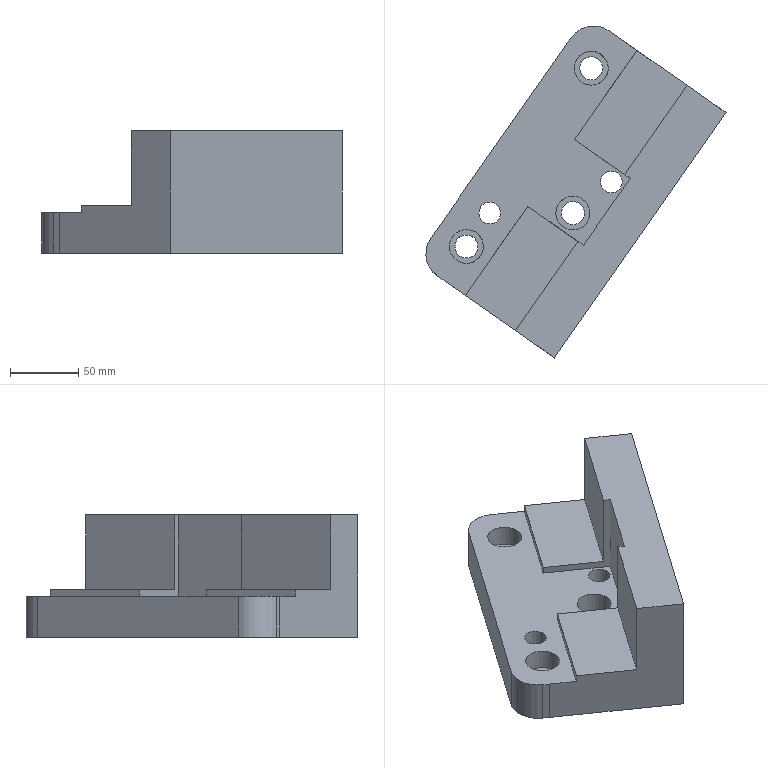Part | NX | features solid 2 | 1 solid | 35 faces | box 220.726 x 244.056 x 90 mm | volume 1242113 mm3 | plane 23 | cylinder 12 | commonest cylinder face diameters 17 x3 25 x3 16 x2 20 x2 40 x2
STEP:
#1=CARTESIAN_POINT('',(39.998,94.071,-429.059));
#2=VERTEX_POINT('',#1);
#3=CARTESIAN_POINT('',(3.136,119.882,-429.059));
#4=VERTEX_POINT('',#3);
#5=CARTESIAN_POINT('',(39.998,94.071,-429.059));
#6=DIRECTION('',(-0.8192,0.5736,0.));
#7=VECTOR('',#6,1000.);
#8=LINE('',#5,#7);
#9=EDGE_CURVE('',#2,#4,#8,.T.);
#10=ORIENTED_EDGE('',*,*,#9,.F.);
#11=CARTESIAN_POINT('',(85.884,159.603,-429.059));
#12=VERTEX_POINT('',#11);
#13=CARTESIAN_POINT('',(85.884,159.603,-429.059));
#14=DIRECTION('',(0.5736,0.8192,0.));
#15=VECTOR('',#14,1000.);
#16=LINE('',#13,#15);
#17=EDGE_CURVE('',#12,#2,#16,.F.);
#18=ORIENTED_EDGE('',*,*,#17,.F.);
#19=CARTESIAN_POINT('',(49.022,185.414,-429.059));
#20=VERTEX_POINT('',#19);
#21=CARTESIAN_POINT('',(85.884,159.603,-429.059));
#22=DIRECTION('',(-0.8192,0.5736,0.));
#23=VECTOR('',#22,1000.);
#24=LINE('',#21,#23);
#25=EDGE_CURVE('',#12,#20,#24,.T.);
#26=ORIENTED_EDGE('',*,*,#25,.T.);
#27=CARTESIAN_POINT('',(49.022,185.414,-429.059));
#28=DIRECTION('',(0.5736,0.8192,0.));
#29=VECTOR('',#28,1000.);
#30=LINE('',#27,#29);
#31=EDGE_CURVE('',#20,#4,#30,.F.);
#32=ORIENTED_EDGE('',*,*,#31,.T.);
#33=EDGE_LOOP('',(#10,#18,#26,#32));
#34=FACE_BOUND('',#33,.T.);
#35=CARTESIAN_POINT('',(85.884,159.603,-429.059));
#36=DIRECTION('',(0.,0.,-1.));
#37=DIRECTION('',(-0.5736,-0.8192,0.));
#38=AXIS2_PLACEMENT_3D('',#35,#36,#37);
#39=PLANE('',#38);
#40=ADVANCED_FACE('',(#34),#39,.F.);
#41=CARTESIAN_POINT('',(120.298,208.752,-429.059));
#42=VERTEX_POINT('',#41);
#43=CARTESIAN_POINT('',(83.437,234.563,-429.059));
#44=VERTEX_POINT('',#43);
#45=CARTESIAN_POINT('',(120.298,208.752,-429.059));
#46=DIRECTION('',(-0.8192,0.5736,0.));
#47=VECTOR('',#46,1000.);
#48=LINE('',#45,#47);
#49=EDGE_CURVE('',#42,#44,#48,.T.);
#50=ORIENTED_EDGE('',*,*,#49,.F.);
#51=CARTESIAN_POINT('',(166.185,274.284,-429.059));
#52=VERTEX_POINT('',#51);
#53=CARTESIAN_POINT('',(166.185,274.284,-429.059));
#54=DIRECTION('',(0.5736,0.8192,0.));
#55=VECTOR('',#54,1000.);
#56=LINE('',#53,#55);
#57=EDGE_CURVE('',#52,#42,#56,.F.);
#58=ORIENTED_EDGE('',*,*,#57,.F.);
#59=CARTESIAN_POINT('',(129.323,300.095,-429.059));
#60=VERTEX_POINT('',#59);
#61=CARTESIAN_POINT('',(166.185,274.284,-429.059));
#62=DIRECTION('',(-0.8192,0.5736,0.));
#63=VECTOR('',#62,1000.);
#64=LINE('',#61,#63);
#65=EDGE_CURVE('',#52,#60,#64,.T.);
#66=ORIENTED_EDGE('',*,*,#65,.T.);
#67=CARTESIAN_POINT('',(129.323,300.095,-429.059));
#68=DIRECTION('',(0.5736,0.8192,0.));
#69=VECTOR('',#68,1000.);
#70=LINE('',#67,#69);
#71=EDGE_CURVE('',#60,#44,#70,.F.);
#72=ORIENTED_EDGE('',*,*,#71,.T.);
#73=EDGE_LOOP('',(#50,#58,#66,#72));
#74=FACE_BOUND('',#73,.T.);
#75=CARTESIAN_POINT('',(166.185,274.284,-429.059));
#76=DIRECTION('',(0.,0.,-1.));
#77=DIRECTION('',(-0.5736,-0.8192,0.));
#78=AXIS2_PLACEMENT_3D('',#75,#76,#77);
#79=PLANE('',#78);
#80=ADVANCED_FACE('',(#74),#79,.F.);
#81=CARTESIAN_POINT('',(102.467,203.428,-434.059));
#82=VERTEX_POINT('',#81);
#83=CARTESIAN_POINT('',(110.467,203.428,-434.059));
#84=DIRECTION('',(0.,0.,-1.));
#85=DIRECTION('',(-1.,0.,0.));
#86=AXIS2_PLACEMENT_3D('',#83,#84,#85);
#87=CIRCLE('',#86,8.);
#88=EDGE_CURVE('',#82,#82,#87,.T.);
#89=ORIENTED_EDGE('',*,*,#88,.T.);
#90=EDGE_LOOP('',(#89));
#91=FACE_BOUND('',#90,.T.);
#92=CARTESIAN_POINT('',(13.167,180.502,-434.059));
#93=VERTEX_POINT('',#92);
#94=CARTESIAN_POINT('',(21.167,180.502,-434.059));
#95=DIRECTION('',(0.,0.,-1.));
#96=DIRECTION('',(-1.,0.,0.));
#97=AXIS2_PLACEMENT_3D('',#94,#95,#96);
#98=CIRCLE('',#97,8.);
#99=EDGE_CURVE('',#93,#93,#98,.T.);
#100=ORIENTED_EDGE('',*,*,#99,.T.);
#101=EDGE_LOOP('',(#100));
#102=FACE_BOUND('',#101,.T.);
#103=CARTESIAN_POINT('',(26.079,152.648,-434.059));
#104=VERTEX_POINT('',#103);
#105=CARTESIAN_POINT('',(3.136,119.882,-434.059));
#106=VERTEX_POINT('',#105);
#107=CARTESIAN_POINT('',(49.022,185.414,-434.059));
#108=DIRECTION('',(-0.5736,-0.8192,0.));
#109=VECTOR('',#108,1000.);
#110=LINE('',#107,#109);
#111=EDGE_CURVE('',#104,#106,#110,.T.);
#112=ORIENTED_EDGE('',*,*,#111,.F.);
#113=CARTESIAN_POINT('',(15.84,159.818,-434.059));
#114=VERTEX_POINT('',#113);
#115=CARTESIAN_POINT('',(26.079,152.648,-434.059));
#116=CARTESIAN_POINT('',(22.666,155.038,-434.059));
#117=CARTESIAN_POINT('',(19.253,157.428,-434.059));
#118=CARTESIAN_POINT('',(15.84,159.818,-434.059));
#119=B_SPLINE_CURVE_WITH_KNOTS('',3,(#115,#116,#117,#118),.UNSPECIFIED.,.F.,.F.,(4,4),(0.,1.25),.UNSPECIFIED.);
#120=EDGE_CURVE('',#104,#114,#119,.T.);
#121=ORIENTED_EDGE('',*,*,#120,.T.);
#122=CARTESIAN_POINT('',(3.96,155.928,-434.059));
#123=DIRECTION('',(0.,0.,-1.));
#124=DIRECTION('',(-1.,0.,0.));
#125=AXIS2_PLACEMENT_3D('',#122,#123,#124);
#126=CIRCLE('',#125,12.5);
#127=EDGE_CURVE('',#114,#114,#126,.T.);
#128=ORIENTED_EDGE('',*,*,#127,.T.);
#129=ORIENTED_EDGE('',*,*,#120,.F.);
#130=CARTESIAN_POINT('',(49.022,185.414,-434.059));
#131=VERTEX_POINT('',#130);
#132=CARTESIAN_POINT('',(49.022,185.414,-434.059));
#133=DIRECTION('',(-0.5736,-0.8192,0.));
#134=VECTOR('',#133,1000.);
#135=LINE('',#132,#134);
#136=EDGE_CURVE('',#131,#104,#135,.T.);
#137=ORIENTED_EDGE('',*,*,#136,.F.);
#138=CARTESIAN_POINT('',(73.597,168.207,-434.059));
#139=VERTEX_POINT('',#138);
#140=CARTESIAN_POINT('',(85.884,159.603,-434.059));
#141=DIRECTION('',(0.8192,-0.5736,0.));
#142=VECTOR('',#141,1000.);
#143=LINE('',#140,#142);
#144=EDGE_CURVE('',#139,#131,#143,.F.);
#145=ORIENTED_EDGE('',*,*,#144,.F.);
#146=CARTESIAN_POINT('',(75.03,170.254,-434.059));
#147=VERTEX_POINT('',#146);
#148=CARTESIAN_POINT('',(73.597,168.207,-434.059));
#149=CARTESIAN_POINT('',(74.074,168.889,-434.059));
#150=CARTESIAN_POINT('',(74.552,169.572,-434.059));
#151=CARTESIAN_POINT('',(75.03,170.254,-434.059));
#152=B_SPLINE_CURVE_WITH_KNOTS('',3,(#148,#149,#150,#151),.UNSPECIFIED.,.F.,.F.,(4,4),(0.,0.5),.UNSPECIFIED.);
#153=EDGE_CURVE('',#139,#147,#152,.T.);
#154=ORIENTED_EDGE('',*,*,#153,.T.);
#155=CARTESIAN_POINT('',(82.2,180.494,-434.059));
#156=DIRECTION('',(0.,0.,-1.));
#157=DIRECTION('',(-1.,0.,0.));
#158=AXIS2_PLACEMENT_3D('',#155,#156,#157);
#159=CIRCLE('',#158,12.5);
#160=EDGE_CURVE('',#147,#147,#159,.T.);
#161=ORIENTED_EDGE('',*,*,#160,.T.);
#162=ORIENTED_EDGE('',*,*,#153,.F.);
#163=CARTESIAN_POINT('',(89.98,156.735,-434.059));
#164=VERTEX_POINT('',#163);
#165=CARTESIAN_POINT('',(85.884,159.603,-434.059));
#166=DIRECTION('',(0.8192,-0.5736,0.));
#167=VECTOR('',#166,1000.);
#168=LINE('',#165,#167);
#169=EDGE_CURVE('',#164,#139,#168,.F.);
#170=ORIENTED_EDGE('',*,*,#169,.F.);
#171=CARTESIAN_POINT('',(124.394,205.884,-434.059));
#172=VERTEX_POINT('',#171);
#173=CARTESIAN_POINT('',(89.98,156.735,-434.059));
#174=DIRECTION('',(-0.5736,-0.8192,0.));
#175=VECTOR('',#174,1000.);
#176=LINE('',#173,#175);
#177=EDGE_CURVE('',#172,#164,#176,.T.);
#178=ORIENTED_EDGE('',*,*,#177,.F.);
#179=CARTESIAN_POINT('',(83.437,234.563,-434.059));
#180=VERTEX_POINT('',#179);
#181=CARTESIAN_POINT('',(120.298,208.752,-434.059));
#182=DIRECTION('',(-0.8192,0.5736,0.));
#183=VECTOR('',#182,1000.);
#184=LINE('',#181,#183);
#185=EDGE_CURVE('',#172,#180,#184,.T.);
#186=ORIENTED_EDGE('',*,*,#185,.T.);
#187=CARTESIAN_POINT('',(112.112,275.516,-434.059));
#188=VERTEX_POINT('',#187);
#189=CARTESIAN_POINT('',(129.323,300.095,-434.059));
#190=DIRECTION('',(-0.5736,-0.8192,0.));
#191=VECTOR('',#190,1000.);
#192=LINE('',#189,#191);
#193=EDGE_CURVE('',#188,#180,#192,.T.);
#194=ORIENTED_EDGE('',*,*,#193,.F.);
#195=CARTESIAN_POINT('',(105.97,279.819,-434.059));
#196=VERTEX_POINT('',#195);
#197=CARTESIAN_POINT('',(112.112,275.516,-434.059));
#198=CARTESIAN_POINT('',(110.064,276.95,-434.059));
#199=CARTESIAN_POINT('',(108.017,278.385,-434.059));
#200=CARTESIAN_POINT('',(105.97,279.819,-434.059));
#201=B_SPLINE_CURVE_WITH_KNOTS('',3,(#197,#198,#199,#200),.UNSPECIFIED.,.F.,.F.,(4,4),(0.,0.75),.UNSPECIFIED.);
#202=EDGE_CURVE('',#196,#188,#201,.F.);
#203=ORIENTED_EDGE('',*,*,#202,.F.);
#204=CARTESIAN_POINT('',(95.732,286.992,-434.059));
#205=DIRECTION('',(0.,0.,-1.));
#206=DIRECTION('',(-1.,0.,0.));
#207=AXIS2_PLACEMENT_3D('',#204,#205,#206);
#208=CIRCLE('',#207,12.5);
#209=EDGE_CURVE('',#196,#196,#208,.T.);
#210=ORIENTED_EDGE('',*,*,#209,.T.);
#211=ORIENTED_EDGE('',*,*,#202,.T.);
#212=CARTESIAN_POINT('',(129.323,300.095,-434.059));
#213=VERTEX_POINT('',#212);
#214=CARTESIAN_POINT('',(129.323,300.095,-434.059));
#215=DIRECTION('',(-0.5736,-0.8192,0.));
#216=VECTOR('',#215,1000.);
#217=LINE('',#214,#216);
#218=EDGE_CURVE('',#213,#188,#217,.T.);
#219=ORIENTED_EDGE('',*,*,#218,.F.);
#220=CARTESIAN_POINT('',(108.844,314.435,-434.059));
#221=VERTEX_POINT('',#220);
#222=CARTESIAN_POINT('',(166.185,274.284,-434.059));
#223=DIRECTION('',(-0.8192,0.5736,0.));
#224=VECTOR('',#223,1000.);
#225=LINE('',#222,#224);
#226=EDGE_CURVE('',#213,#221,#225,.T.);
#227=ORIENTED_EDGE('',*,*,#226,.T.);
#228=CARTESIAN_POINT('',(80.989,309.523,-434.059));
#229=VERTEX_POINT('',#228);
#230=CARTESIAN_POINT('',(97.372,298.052,-434.059));
#231=DIRECTION('',(0.,0.,-1.));
#232=DIRECTION('',(-1.,0.,0.));
#233=AXIS2_PLACEMENT_3D('',#230,#231,#232);
#234=CIRCLE('',#233,20.);
#235=EDGE_CURVE('',#221,#229,#234,.F.);
#236=ORIENTED_EDGE('',*,*,#235,.T.);
#237=CARTESIAN_POINT('',(-22.254,162.076,-434.059));
#238=VERTEX_POINT('',#237);
#239=CARTESIAN_POINT('',(12.16,211.225,-434.059));
#240=DIRECTION('',(-0.5736,-0.8192,0.));
#241=VECTOR('',#240,1000.);
#242=LINE('',#239,#241);
#243=EDGE_CURVE('',#229,#238,#242,.T.);
#244=ORIENTED_EDGE('',*,*,#243,.T.);
#245=CARTESIAN_POINT('',(-17.343,134.221,-434.059));
#246=VERTEX_POINT('',#245);
#247=CARTESIAN_POINT('',(-5.871,150.604,-434.059));
#248=DIRECTION('',(0.,0.,-1.));
#249=DIRECTION('',(-1.,0.,0.));
#250=AXIS2_PLACEMENT_3D('',#247,#248,#249);
#251=CIRCLE('',#250,20.);
#252=EDGE_CURVE('',#238,#246,#251,.F.);
#253=ORIENTED_EDGE('',*,*,#252,.T.);
#254=CARTESIAN_POINT('',(-13.247,131.353,-434.059));
#255=VERTEX_POINT('',#254);
#256=CARTESIAN_POINT('',(27.71,102.674,-434.059));
#257=DIRECTION('',(0.8192,-0.5736,0.));
#258=VECTOR('',#257,1000.);
#259=LINE('',#256,#258);
#260=EDGE_CURVE('',#246,#255,#259,.T.);
#261=ORIENTED_EDGE('',*,*,#260,.T.);
#262=CARTESIAN_POINT('',(39.998,94.071,-434.059));
#263=DIRECTION('',(0.8192,-0.5736,0.));
#264=VECTOR('',#263,1000.);
#265=LINE('',#262,#264);
#266=EDGE_CURVE('',#255,#106,#265,.T.);
#267=ORIENTED_EDGE('',*,*,#266,.T.);
#268=EDGE_LOOP('',(#112,#121,#128,#129,#137,#145,#154,#161,#162,#170,#178,#186,#194,#203,#210,#211,#219,#227,#236,#244,#253,#261,#267));
#269=FACE_BOUND('',#268,.T.);
#270=CARTESIAN_POINT('',(85.884,159.603,-434.059));
#271=DIRECTION('',(0.,0.,-1.));
#272=DIRECTION('',(-0.5736,-0.8192,0.));
#273=AXIS2_PLACEMENT_3D('',#270,#271,#272);
#274=PLANE('',#273);
#275=ADVANCED_FACE('',(#91,#102,#269),#274,.F.);
#276=CARTESIAN_POINT('',(194.855,254.209,-464.059));
#277=VERTEX_POINT('',#276);
#278=CARTESIAN_POINT('',(108.844,314.435,-464.059));
#279=VERTEX_POINT('',#278);
#280=CARTESIAN_POINT('',(166.185,274.284,-464.059));
#281=DIRECTION('',(-0.8192,0.5736,0.));
#282=VECTOR('',#281,1000.);
#283=LINE('',#280,#282);
#284=EDGE_CURVE('',#277,#279,#283,.T.);
#285=ORIENTED_EDGE('',*,*,#284,.T.);
#286=CARTESIAN_POINT('',(108.844,314.435,-439.059));
#287=DIRECTION('',(0.,0.,-1.));
#288=VECTOR('',#287,1000.);
#289=LINE('',#286,#288);
#290=EDGE_CURVE('',#279,#221,#289,.F.);
#291=ORIENTED_EDGE('',*,*,#290,.T.);
#292=ORIENTED_EDGE('',*,*,#226,.F.);
#293=CARTESIAN_POINT('',(129.323,300.095,-439.059));
#294=DIRECTION('',(0.,0.,1.));
#295=VECTOR('',#294,1000.);
#296=LINE('',#293,#295);
#297=EDGE_CURVE('',#213,#60,#296,.T.);
#298=ORIENTED_EDGE('',*,*,#297,.T.);
#299=ORIENTED_EDGE('',*,*,#65,.F.);
#300=CARTESIAN_POINT('',(166.185,274.284,-374.059));
#301=VERTEX_POINT('',#300);
#302=CARTESIAN_POINT('',(166.185,274.284,-369.059));
#303=DIRECTION('',(0.,0.,1.));
#304=VECTOR('',#303,1000.);
#305=LINE('',#302,#304);
#306=EDGE_CURVE('',#301,#52,#305,.F.);
#307=ORIENTED_EDGE('',*,*,#306,.F.);
#308=CARTESIAN_POINT('',(194.855,254.209,-374.059));
#309=VERTEX_POINT('',#308);
#310=CARTESIAN_POINT('',(133.418,297.227,-374.059));
#311=DIRECTION('',(-0.8192,0.5736,0.));
#312=VECTOR('',#311,1000.);
#313=LINE('',#310,#312);
#314=EDGE_CURVE('',#301,#309,#313,.F.);
#315=ORIENTED_EDGE('',*,*,#314,.T.);
#316=CARTESIAN_POINT('',(194.855,254.209,-475.));
#317=DIRECTION('',(0.,0.,-1.));
#318=VECTOR('',#317,1000.);
#319=LINE('',#316,#318);
#320=EDGE_CURVE('',#309,#277,#319,.T.);
#321=ORIENTED_EDGE('',*,*,#320,.T.);
#322=EDGE_LOOP('',(#285,#291,#292,#298,#299,#307,#315,#321));
#323=FACE_BOUND('',#322,.T.);
#324=CARTESIAN_POINT('',(166.185,274.284,-439.059));
#325=DIRECTION('',(-0.5736,-0.8192,0.));
#326=DIRECTION('',(0.,0.,1.));
#327=AXIS2_PLACEMENT_3D('',#324,#325,#326);
#328=PLANE('',#327);
#329=ADVANCED_FACE('',(#323),#328,.F.);
#330=CARTESIAN_POINT('',(3.136,119.882,-439.059));
#331=DIRECTION('',(0.,0.,1.));
#332=VECTOR('',#331,1000.);
#333=LINE('',#330,#332);
#334=EDGE_CURVE('',#106,#4,#333,.T.);
#335=ORIENTED_EDGE('',*,*,#334,.F.);
#336=ORIENTED_EDGE('',*,*,#266,.F.);
#337=CARTESIAN_POINT('',(-13.247,131.353,-464.059));
#338=VERTEX_POINT('',#337);
#339=CARTESIAN_POINT('',(-13.247,131.353,-469.059));
#340=DIRECTION('',(0.,0.,-1.));
#341=VECTOR('',#340,1000.);
#342=LINE('',#339,#341);
#343=EDGE_CURVE('',#255,#338,#342,.T.);
#344=ORIENTED_EDGE('',*,*,#343,.T.);
#345=CARTESIAN_POINT('',(68.668,73.996,-464.059));
#346=VERTEX_POINT('',#345);
#347=CARTESIAN_POINT('',(39.998,94.071,-464.059));
#348=DIRECTION('',(-0.8192,0.5736,0.));
#349=VECTOR('',#348,1000.);
#350=LINE('',#347,#349);
#351=EDGE_CURVE('',#346,#338,#350,.T.);
#352=ORIENTED_EDGE('',*,*,#351,.F.);
#353=CARTESIAN_POINT('',(68.668,73.996,-374.059));
#354=VERTEX_POINT('',#353);
#355=CARTESIAN_POINT('',(68.668,73.996,-475.));
#356=DIRECTION('',(0.,0.,-1.));
#357=VECTOR('',#356,1000.);
#358=LINE('',#355,#357);
#359=EDGE_CURVE('',#354,#346,#358,.T.);
#360=ORIENTED_EDGE('',*,*,#359,.F.);
#361=CARTESIAN_POINT('',(39.998,94.071,-374.059));
#362=VERTEX_POINT('',#361);
#363=CARTESIAN_POINT('',(7.232,117.014,-374.059));
#364=DIRECTION('',(-0.8192,0.5736,0.));
#365=VECTOR('',#364,1000.);
#366=LINE('',#363,#365);
#367=EDGE_CURVE('',#362,#354,#366,.F.);
#368=ORIENTED_EDGE('',*,*,#367,.F.);
#369=CARTESIAN_POINT('',(39.998,94.071,-369.059));
#370=DIRECTION('',(0.,0.,1.));
#371=VECTOR('',#370,1000.);
#372=LINE('',#369,#371);
#373=EDGE_CURVE('',#362,#2,#372,.F.);
#374=ORIENTED_EDGE('',*,*,#373,.T.);
#375=ORIENTED_EDGE('',*,*,#9,.T.);
#376=EDGE_LOOP('',(#335,#336,#344,#352,#360,#368,#374,#375));
#377=FACE_BOUND('',#376,.T.);
#378=CARTESIAN_POINT('',(39.998,94.071,-439.059));
#379=DIRECTION('',(-0.5736,-0.8192,0.));
#380=DIRECTION('',(0.8192,-0.5736,0.));
#381=AXIS2_PLACEMENT_3D('',#378,#379,#380);
#382=PLANE('',#381);
#383=ADVANCED_FACE('',(#377),#382,.T.);
#384=ORIENTED_EDGE('',*,*,#243,.F.);
#385=CARTESIAN_POINT('',(80.989,309.523,-464.059));
#386=VERTEX_POINT('',#385);
#387=CARTESIAN_POINT('',(80.989,309.523,-439.059));
#388=DIRECTION('',(0.,0.,-1.));
#389=VECTOR('',#388,1000.);
#390=LINE('',#387,#389);
#391=EDGE_CURVE('',#229,#386,#390,.T.);
#392=ORIENTED_EDGE('',*,*,#391,.T.);
#393=CARTESIAN_POINT('',(-22.254,162.076,-464.059));
#394=VERTEX_POINT('',#393);
#395=CARTESIAN_POINT('',(12.16,211.225,-464.059));
#396=DIRECTION('',(-0.5736,-0.8192,0.));
#397=VECTOR('',#396,1000.);
#398=LINE('',#395,#397);
#399=EDGE_CURVE('',#386,#394,#398,.T.);
#400=ORIENTED_EDGE('',*,*,#399,.T.);
#401=CARTESIAN_POINT('',(-22.254,162.076,-434.059));
#402=DIRECTION('',(0.,0.,1.));
#403=VECTOR('',#402,1000.);
#404=LINE('',#401,#403);
#405=EDGE_CURVE('',#394,#238,#404,.T.);
#406=ORIENTED_EDGE('',*,*,#405,.T.);
#407=EDGE_LOOP('',(#384,#392,#400,#406));
#408=FACE_BOUND('',#407,.T.);
#409=CARTESIAN_POINT('',(12.16,211.225,-439.059));
#410=DIRECTION('',(0.8192,-0.5736,0.));
#411=DIRECTION('',(0.5736,0.8192,0.));
#412=AXIS2_PLACEMENT_3D('',#409,#410,#411);
#413=PLANE('',#412);
#414=ADVANCED_FACE('',(#408),#413,.F.);
#415=CARTESIAN_POINT('',(85.892,220.636,-464.059));
#416=VERTEX_POINT('',#415);
#417=CARTESIAN_POINT('',(62.949,187.87,-464.059));
#418=VERTEX_POINT('',#417);
#419=CARTESIAN_POINT('',(57.213,179.678,-464.059));
#420=DIRECTION('',(-0.5736,-0.8192,0.));
#421=VECTOR('',#420,1000.);
#422=LINE('',#419,#421);
#423=EDGE_CURVE('',#416,#418,#422,.T.);
#424=ORIENTED_EDGE('',*,*,#423,.F.);
#425=CARTESIAN_POINT('',(69.509,232.107,-464.059));
#426=VERTEX_POINT('',#425);
#427=CARTESIAN_POINT('',(77.701,226.371,-464.059));
#428=DIRECTION('',(0.,0.,-1.));
#429=DIRECTION('',(-1.,0.,0.));
#430=AXIS2_PLACEMENT_3D('',#427,#428,#429);
#431=CIRCLE('',#430,10.);
#432=EDGE_CURVE('',#416,#426,#431,.F.);
#433=ORIENTED_EDGE('',*,*,#432,.T.);
#434=CARTESIAN_POINT('',(46.566,199.341,-464.059));
#435=VERTEX_POINT('',#434);
#436=CARTESIAN_POINT('',(40.83,191.15,-464.059));
#437=DIRECTION('',(-0.5736,-0.8192,0.));
#438=VECTOR('',#437,1000.);
#439=LINE('',#436,#438);
#440=EDGE_CURVE('',#426,#435,#439,.T.);
#441=ORIENTED_EDGE('',*,*,#440,.T.);
#442=CARTESIAN_POINT('',(54.758,193.605,-464.059));
#443=DIRECTION('',(0.,0.,-1.));
#444=DIRECTION('',(-1.,0.,0.));
#445=AXIS2_PLACEMENT_3D('',#442,#443,#444);
#446=CIRCLE('',#445,10.);
#447=EDGE_CURVE('',#435,#418,#446,.F.);
#448=ORIENTED_EDGE('',*,*,#447,.T.);
#449=EDGE_LOOP('',(#424,#433,#441,#448));
#450=FACE_BOUND('',#449,.T.);
#451=CARTESIAN_POINT('',(102.467,203.428,-464.059));
#452=VERTEX_POINT('',#451);
#453=CARTESIAN_POINT('',(110.467,203.428,-464.059));
#454=DIRECTION('',(0.,0.,-1.));
#455=DIRECTION('',(-1.,0.,0.));
#456=AXIS2_PLACEMENT_3D('',#453,#454,#455);
#457=CIRCLE('',#456,8.);
#458=EDGE_CURVE('',#452,#452,#457,.T.);
#459=ORIENTED_EDGE('',*,*,#458,.F.);
#460=EDGE_LOOP('',(#459));
#461=FACE_BOUND('',#460,.T.);
#462=CARTESIAN_POINT('',(13.167,180.502,-464.059));
#463=VERTEX_POINT('',#462);
#464=CARTESIAN_POINT('',(21.167,180.502,-464.059));
#465=DIRECTION('',(0.,0.,-1.));
#466=DIRECTION('',(-1.,0.,0.));
#467=AXIS2_PLACEMENT_3D('',#464,#465,#466);
#468=CIRCLE('',#467,8.);
#469=EDGE_CURVE('',#463,#463,#468,.T.);
#470=ORIENTED_EDGE('',*,*,#469,.F.);
#471=EDGE_LOOP('',(#470));
#472=FACE_BOUND('',#471,.T.);
#473=CARTESIAN_POINT('',(73.7,180.494,-464.059));
#474=VERTEX_POINT('',#473);
#475=CARTESIAN_POINT('',(82.2,180.494,-464.059));
#476=DIRECTION('',(0.,0.,-1.));
#477=DIRECTION('',(-1.,0.,0.));
#478=AXIS2_PLACEMENT_3D('',#475,#476,#477);
#479=CIRCLE('',#478,8.5);
#480=EDGE_CURVE('',#474,#474,#479,.T.);
#481=ORIENTED_EDGE('',*,*,#480,.F.);
#482=EDGE_LOOP('',(#481));
#483=FACE_BOUND('',#482,.T.);
#484=CARTESIAN_POINT('',(-4.54,155.928,-464.059));
#485=VERTEX_POINT('',#484);
#486=CARTESIAN_POINT('',(3.96,155.928,-464.059));
#487=DIRECTION('',(0.,0.,-1.));
#488=DIRECTION('',(-1.,0.,0.));
#489=AXIS2_PLACEMENT_3D('',#486,#487,#488);
#490=CIRCLE('',#489,8.5);
#491=EDGE_CURVE('',#485,#485,#490,.T.);
#492=ORIENTED_EDGE('',*,*,#491,.F.);
#493=EDGE_LOOP('',(#492));
#494=FACE_BOUND('',#493,.T.);
#495=CARTESIAN_POINT('',(87.232,286.992,-464.059));
#496=VERTEX_POINT('',#495);
#497=CARTESIAN_POINT('',(95.732,286.992,-464.059));
#498=DIRECTION('',(0.,0.,-1.));
#499=DIRECTION('',(-1.,0.,0.));
#500=AXIS2_PLACEMENT_3D('',#497,#498,#499);
#501=CIRCLE('',#500,8.5);
#502=EDGE_CURVE('',#496,#496,#501,.T.);
#503=ORIENTED_EDGE('',*,*,#502,.F.);
#504=EDGE_LOOP('',(#503));
#505=FACE_BOUND('',#504,.T.);
#506=ORIENTED_EDGE('',*,*,#399,.F.);
#507=CARTESIAN_POINT('',(97.372,298.052,-464.059));
#508=DIRECTION('',(0.,0.,-1.));
#509=DIRECTION('',(-1.,0.,0.));
#510=AXIS2_PLACEMENT_3D('',#507,#508,#509);
#511=CIRCLE('',#510,20.);
#512=EDGE_CURVE('',#386,#279,#511,.T.);
#513=ORIENTED_EDGE('',*,*,#512,.T.);
#514=ORIENTED_EDGE('',*,*,#284,.F.);
#515=CARTESIAN_POINT('',(114.554,139.528,-464.059));
#516=DIRECTION('',(-0.5736,-0.8192,0.));
#517=VECTOR('',#516,1000.);
#518=LINE('',#515,#517);
#519=EDGE_CURVE('',#277,#346,#518,.T.);
#520=ORIENTED_EDGE('',*,*,#519,.T.);
#521=ORIENTED_EDGE('',*,*,#351,.T.);
#522=CARTESIAN_POINT('',(-17.343,134.221,-464.059));
#523=VERTEX_POINT('',#522);
#524=CARTESIAN_POINT('',(27.71,102.674,-464.059));
#525=DIRECTION('',(-0.8192,0.5736,0.));
#526=VECTOR('',#525,1000.);
#527=LINE('',#524,#526);
#528=EDGE_CURVE('',#338,#523,#527,.T.);
#529=ORIENTED_EDGE('',*,*,#528,.T.);
#530=CARTESIAN_POINT('',(-5.871,150.604,-464.059));
#531=DIRECTION('',(0.,0.,-1.));
#532=DIRECTION('',(-1.,0.,0.));
#533=AXIS2_PLACEMENT_3D('',#530,#531,#532);
#534=CIRCLE('',#533,20.);
#535=EDGE_CURVE('',#523,#394,#534,.T.);
#536=ORIENTED_EDGE('',*,*,#535,.T.);
#537=EDGE_LOOP('',(#506,#513,#514,#520,#521,#529,#536));
#538=FACE_BOUND('',#537,.T.);
#539=CARTESIAN_POINT('',(85.884,159.603,-464.059));
#540=DIRECTION('',(0.,0.,-1.));
#541=DIRECTION('',(-0.5736,-0.8192,0.));
#542=AXIS2_PLACEMENT_3D('',#539,#540,#541);
#543=PLANE('',#542);
#544=ADVANCED_FACE('',(#450,#461,#472,#483,#494,#505,#538),#543,.T.);
#545=ORIENTED_EDGE('',*,*,#31,.F.);
#546=CARTESIAN_POINT('',(49.022,185.414,-439.059));
#547=DIRECTION('',(0.,0.,-1.));
#548=VECTOR('',#547,1000.);
#549=LINE('',#546,#548);
#550=EDGE_CURVE('',#131,#20,#549,.F.);
#551=ORIENTED_EDGE('',*,*,#550,.F.);
#552=ORIENTED_EDGE('',*,*,#136,.T.);
#553=ORIENTED_EDGE('',*,*,#111,.T.);
#554=ORIENTED_EDGE('',*,*,#334,.T.);
#555=EDGE_LOOP('',(#545,#551,#552,#553,#554));
#556=FACE_BOUND('',#555,.T.);
#557=CARTESIAN_POINT('',(49.022,185.414,-439.059));
#558=DIRECTION('',(-0.8192,0.5736,0.));
#559=DIRECTION('',(-0.5736,-0.8192,0.));
#560=AXIS2_PLACEMENT_3D('',#557,#558,#559);
#561=PLANE('',#560);
#562=ADVANCED_FACE('',(#556),#561,.T.);
#563=CARTESIAN_POINT('',(89.98,156.735,-374.059));
#564=VERTEX_POINT('',#563);
#565=CARTESIAN_POINT('',(89.98,156.735,-439.059));
#566=DIRECTION('',(0.,0.,-1.));
#567=VECTOR('',#566,1000.);
#568=LINE('',#565,#567);
#569=EDGE_CURVE('',#164,#564,#568,.F.);
#570=ORIENTED_EDGE('',*,*,#569,.F.);
#571=ORIENTED_EDGE('',*,*,#169,.T.);
#572=ORIENTED_EDGE('',*,*,#144,.T.);
#573=ORIENTED_EDGE('',*,*,#550,.T.);
#574=ORIENTED_EDGE('',*,*,#25,.F.);
#575=CARTESIAN_POINT('',(85.884,159.603,-374.059));
#576=VERTEX_POINT('',#575);
#577=CARTESIAN_POINT('',(85.884,159.603,-369.059));
#578=DIRECTION('',(0.,0.,1.));
#579=VECTOR('',#578,1000.);
#580=LINE('',#577,#579);
#581=EDGE_CURVE('',#576,#12,#580,.F.);
#582=ORIENTED_EDGE('',*,*,#581,.F.);
#583=CARTESIAN_POINT('',(53.118,182.546,-374.059));
#584=DIRECTION('',(-0.8192,0.5736,0.));
#585=VECTOR('',#584,1000.);
#586=LINE('',#583,#585);
#587=EDGE_CURVE('',#564,#576,#586,.T.);
#588=ORIENTED_EDGE('',*,*,#587,.F.);
#589=EDGE_LOOP('',(#570,#571,#572,#573,#574,#582,#588));
#590=FACE_BOUND('',#589,.T.);
#591=CARTESIAN_POINT('',(85.884,159.603,-439.059));
#592=DIRECTION('',(-0.5736,-0.8192,0.));
#593=DIRECTION('',(0.,0.,1.));
#594=AXIS2_PLACEMENT_3D('',#591,#592,#593);
#595=PLANE('',#594);
#596=ADVANCED_FACE('',(#590),#595,.F.);
#597=ORIENTED_EDGE('',*,*,#185,.F.);
#598=CARTESIAN_POINT('',(124.394,205.884,-374.059));
#599=VERTEX_POINT('',#598);
#600=CARTESIAN_POINT('',(124.394,205.884,-439.059));
#601=DIRECTION('',(0.,0.,1.));
#602=VECTOR('',#601,1000.);
#603=LINE('',#600,#602);
#604=EDGE_CURVE('',#172,#599,#603,.T.);
#605=ORIENTED_EDGE('',*,*,#604,.T.);
#606=CARTESIAN_POINT('',(120.298,208.752,-374.059));
#607=VERTEX_POINT('',#606);
#608=CARTESIAN_POINT('',(120.298,208.752,-374.059));
#609=DIRECTION('',(0.8192,-0.5736,0.));
#610=VECTOR('',#609,1000.);
#611=LINE('',#608,#610);
#612=EDGE_CURVE('',#599,#607,#611,.F.);
#613=ORIENTED_EDGE('',*,*,#612,.T.);
#614=CARTESIAN_POINT('',(120.298,208.752,-369.059));
#615=DIRECTION('',(0.,0.,1.));
#616=VECTOR('',#615,1000.);
#617=LINE('',#614,#616);
#618=EDGE_CURVE('',#607,#42,#617,.F.);
#619=ORIENTED_EDGE('',*,*,#618,.T.);
#620=ORIENTED_EDGE('',*,*,#49,.T.);
#621=CARTESIAN_POINT('',(83.437,234.563,-439.059));
#622=DIRECTION('',(0.,0.,1.));
#623=VECTOR('',#622,1000.);
#624=LINE('',#621,#623);
#625=EDGE_CURVE('',#180,#44,#624,.T.);
#626=ORIENTED_EDGE('',*,*,#625,.F.);
#627=EDGE_LOOP('',(#597,#605,#613,#619,#620,#626));
#628=FACE_BOUND('',#627,.T.);
#629=CARTESIAN_POINT('',(120.298,208.752,-439.059));
#630=DIRECTION('',(-0.5736,-0.8192,0.));
#631=DIRECTION('',(0.,0.,1.));
#632=AXIS2_PLACEMENT_3D('',#629,#630,#631);
#633=PLANE('',#632);
#634=ADVANCED_FACE('',(#628),#633,.T.);
#635=ORIENTED_EDGE('',*,*,#71,.F.);
#636=ORIENTED_EDGE('',*,*,#297,.F.);
#637=ORIENTED_EDGE('',*,*,#218,.T.);
#638=ORIENTED_EDGE('',*,*,#193,.T.);
#639=ORIENTED_EDGE('',*,*,#625,.T.);
#640=EDGE_LOOP('',(#635,#636,#637,#638,#639));
#641=FACE_BOUND('',#640,.T.);
#642=CARTESIAN_POINT('',(129.323,300.095,-439.059));
#643=DIRECTION('',(-0.8192,0.5736,0.));
#644=DIRECTION('',(-0.5736,-0.8192,0.));
#645=AXIS2_PLACEMENT_3D('',#642,#643,#644);
#646=PLANE('',#645);
#647=ADVANCED_FACE('',(#641),#646,.T.);
#648=CARTESIAN_POINT('',(171.912,221.443,-374.059));
#649=DIRECTION('',(0.5736,0.8192,0.));
#650=VECTOR('',#649,1000.);
#651=LINE('',#648,#650);
#652=EDGE_CURVE('',#309,#354,#651,.F.);
#653=ORIENTED_EDGE('',*,*,#652,.F.);
#654=ORIENTED_EDGE('',*,*,#314,.F.);
#655=CARTESIAN_POINT('',(166.185,274.284,-374.059));
#656=DIRECTION('',(0.5736,0.8192,0.));
#657=VECTOR('',#656,1000.);
#658=LINE('',#655,#657);
#659=EDGE_CURVE('',#301,#607,#658,.F.);
#660=ORIENTED_EDGE('',*,*,#659,.T.);
#661=ORIENTED_EDGE('',*,*,#612,.F.);
#662=CARTESIAN_POINT('',(89.98,156.735,-374.059));
#663=DIRECTION('',(0.5736,0.8192,0.));
#664=VECTOR('',#663,1000.);
#665=LINE('',#662,#664);
#666=EDGE_CURVE('',#599,#564,#665,.F.);
#667=ORIENTED_EDGE('',*,*,#666,.T.);
#668=ORIENTED_EDGE('',*,*,#587,.T.);
#669=CARTESIAN_POINT('',(85.884,159.603,-374.059));
#670=DIRECTION('',(0.5736,0.8192,0.));
#671=VECTOR('',#670,1000.);
#672=LINE('',#669,#671);
#673=EDGE_CURVE('',#576,#362,#672,.F.);
#674=ORIENTED_EDGE('',*,*,#673,.T.);
#675=ORIENTED_EDGE('',*,*,#367,.T.);
#676=EDGE_LOOP('',(#653,#654,#660,#661,#667,#668,#674,#675));
#677=FACE_BOUND('',#676,.T.);
#678=CARTESIAN_POINT('',(130.551,293.132,-374.059));
#679=DIRECTION('',(0.,0.,-1.));
#680=DIRECTION('',(-0.8192,0.5736,0.));
#681=AXIS2_PLACEMENT_3D('',#678,#679,#680);
#682=PLANE('',#681);
#683=ADVANCED_FACE('',(#677),#682,.F.);
#684=ORIENTED_EDGE('',*,*,#569,.T.);
#685=ORIENTED_EDGE('',*,*,#666,.F.);
#686=ORIENTED_EDGE('',*,*,#604,.F.);
#687=ORIENTED_EDGE('',*,*,#177,.T.);
#688=EDGE_LOOP('',(#684,#685,#686,#687));
#689=FACE_BOUND('',#688,.T.);
#690=CARTESIAN_POINT('',(89.98,156.735,-439.059));
#691=DIRECTION('',(0.8192,-0.5736,0.));
#692=DIRECTION('',(0.5736,0.8192,0.));
#693=AXIS2_PLACEMENT_3D('',#690,#691,#692);
#694=PLANE('',#693);
#695=ADVANCED_FACE('',(#689),#694,.F.);
#696=ORIENTED_EDGE('',*,*,#519,.F.);
#697=ORIENTED_EDGE('',*,*,#320,.F.);
#698=ORIENTED_EDGE('',*,*,#652,.T.);
#699=ORIENTED_EDGE('',*,*,#359,.T.);
#700=EDGE_LOOP('',(#696,#697,#698,#699));
#701=FACE_BOUND('',#700,.T.);
#702=CARTESIAN_POINT('',(171.912,221.443,-475.));
#703=DIRECTION('',(0.8192,-0.5736,0.));
#704=DIRECTION('',(0.,0.,-1.));
#705=AXIS2_PLACEMENT_3D('',#702,#703,#704);
#706=PLANE('',#705);
#707=ADVANCED_FACE('',(#701),#706,.T.);
#708=ORIENTED_EDGE('',*,*,#57,.T.);
#709=ORIENTED_EDGE('',*,*,#618,.F.);
#710=ORIENTED_EDGE('',*,*,#659,.F.);
#711=ORIENTED_EDGE('',*,*,#306,.T.);
#712=EDGE_LOOP('',(#708,#709,#710,#711));
#713=FACE_BOUND('',#712,.T.);
#714=CARTESIAN_POINT('',(166.185,274.284,-369.059));
#715=DIRECTION('',(0.8192,-0.5736,0.));
#716=DIRECTION('',(0.5736,0.8192,0.));
#717=AXIS2_PLACEMENT_3D('',#714,#715,#716);
#718=PLANE('',#717);
#719=ADVANCED_FACE('',(#713),#718,.F.);
#720=ORIENTED_EDGE('',*,*,#17,.T.);
#721=ORIENTED_EDGE('',*,*,#373,.F.);
#722=ORIENTED_EDGE('',*,*,#673,.F.);
#723=ORIENTED_EDGE('',*,*,#581,.T.);
#724=EDGE_LOOP('',(#720,#721,#722,#723));
#725=FACE_BOUND('',#724,.T.);
#726=CARTESIAN_POINT('',(85.884,159.603,-369.059));
#727=DIRECTION('',(0.8192,-0.5736,0.));
#728=DIRECTION('',(0.5736,0.8192,0.));
#729=AXIS2_PLACEMENT_3D('',#726,#727,#728);
#730=PLANE('',#729);
#731=ADVANCED_FACE('',(#725),#730,.F.);
#732=ORIENTED_EDGE('',*,*,#260,.F.);
#733=CARTESIAN_POINT('',(-17.343,134.221,-469.059));
#734=DIRECTION('',(0.,0.,1.));
#735=VECTOR('',#734,1000.);
#736=LINE('',#733,#735);
#737=EDGE_CURVE('',#246,#523,#736,.F.);
#738=ORIENTED_EDGE('',*,*,#737,.T.);
#739=ORIENTED_EDGE('',*,*,#528,.F.);
#740=ORIENTED_EDGE('',*,*,#343,.F.);
#741=EDGE_LOOP('',(#732,#738,#739,#740));
#742=FACE_BOUND('',#741,.T.);
#743=CARTESIAN_POINT('',(27.71,102.674,-439.059));
#744=DIRECTION('',(-0.5736,-0.8192,0.));
#745=DIRECTION('',(0.8192,-0.5736,0.));
#746=AXIS2_PLACEMENT_3D('',#743,#744,#745);
#747=PLANE('',#746);
#748=ADVANCED_FACE('',(#742),#747,.T.);
#749=ORIENTED_EDGE('',*,*,#535,.F.);
#750=ORIENTED_EDGE('',*,*,#737,.F.);
#751=ORIENTED_EDGE('',*,*,#252,.F.);
#752=ORIENTED_EDGE('',*,*,#405,.F.);
#753=EDGE_LOOP('',(#749,#750,#751,#752));
#754=FACE_BOUND('',#753,.T.);
#755=CARTESIAN_POINT('',(-5.871,150.604,-439.059));
#756=DIRECTION('',(0.,0.,-1.));
#757=DIRECTION('',(-1.,0.,0.));
#758=AXIS2_PLACEMENT_3D('',#755,#756,#757);
#759=CYLINDRICAL_SURFACE('',#758,20.);
#760=ADVANCED_FACE('',(#754),#759,.T.);
#761=ORIENTED_EDGE('',*,*,#235,.F.);
#762=ORIENTED_EDGE('',*,*,#290,.F.);
#763=ORIENTED_EDGE('',*,*,#512,.F.);
#764=ORIENTED_EDGE('',*,*,#391,.F.);
#765=EDGE_LOOP('',(#761,#762,#763,#764));
#766=FACE_BOUND('',#765,.T.);
#767=CARTESIAN_POINT('',(97.372,298.052,-439.059));
#768=DIRECTION('',(0.,0.,-1.));
#769=DIRECTION('',(-1.,0.,0.));
#770=AXIS2_PLACEMENT_3D('',#767,#768,#769);
#771=CYLINDRICAL_SURFACE('',#770,20.);
#772=ADVANCED_FACE('',(#766),#771,.T.);
#773=ORIENTED_EDGE('',*,*,#502,.T.);
#774=EDGE_LOOP('',(#773));
#775=FACE_BOUND('',#774,.T.);
#776=CARTESIAN_POINT('',(87.232,286.992,-449.059));
#777=VERTEX_POINT('',#776);
#778=CARTESIAN_POINT('',(95.732,286.992,-449.059));
#779=DIRECTION('',(0.,0.,-1.));
#780=DIRECTION('',(-1.,0.,0.));
#781=AXIS2_PLACEMENT_3D('',#778,#779,#780);
#782=CIRCLE('',#781,8.5);
#783=EDGE_CURVE('',#777,#777,#782,.T.);
#784=ORIENTED_EDGE('',*,*,#783,.F.);
#785=EDGE_LOOP('',(#784));
#786=FACE_BOUND('',#785,.T.);
#787=CARTESIAN_POINT('',(95.732,286.992,-484.059));
#788=DIRECTION('',(0.,0.,-1.));
#789=DIRECTION('',(-1.,0.,0.));
#790=AXIS2_PLACEMENT_3D('',#787,#788,#789);
#791=CYLINDRICAL_SURFACE('',#790,8.5);
#792=ADVANCED_FACE('',(#775,#786),#791,.F.);
#793=ORIENTED_EDGE('',*,*,#783,.T.);
#794=EDGE_LOOP('',(#793));
#795=FACE_BOUND('',#794,.T.);
#796=CARTESIAN_POINT('',(83.232,286.992,-449.059));
#797=VERTEX_POINT('',#796);
#798=CARTESIAN_POINT('',(95.732,286.992,-449.059));
#799=DIRECTION('',(0.,0.,-1.));
#800=DIRECTION('',(-1.,0.,0.));
#801=AXIS2_PLACEMENT_3D('',#798,#799,#800);
#802=CIRCLE('',#801,12.5);
#803=EDGE_CURVE('',#797,#797,#802,.T.);
#804=ORIENTED_EDGE('',*,*,#803,.F.);
#805=EDGE_LOOP('',(#804));
#806=FACE_BOUND('',#805,.T.);
#807=CARTESIAN_POINT('',(94.092,275.933,-449.059));
#808=DIRECTION('',(0.,0.,-1.));
#809=DIRECTION('',(-1.,0.,0.));
#810=AXIS2_PLACEMENT_3D('',#807,#808,#809);
#811=PLANE('',#810);
#812=ADVANCED_FACE('',(#795,#806),#811,.F.);
#813=ORIENTED_EDGE('',*,*,#803,.T.);
#814=EDGE_LOOP('',(#813));
#815=FACE_BOUND('',#814,.T.);
#816=ORIENTED_EDGE('',*,*,#209,.F.);
#817=EDGE_LOOP('',(#816));
#818=FACE_BOUND('',#817,.T.);
#819=CARTESIAN_POINT('',(95.732,286.992,-434.059));
#820=DIRECTION('',(0.,0.,-1.));
#821=DIRECTION('',(-1.,0.,0.));
#822=AXIS2_PLACEMENT_3D('',#819,#820,#821);
#823=CYLINDRICAL_SURFACE('',#822,12.5);
#824=ADVANCED_FACE('',(#815,#818),#823,.F.);
#825=ORIENTED_EDGE('',*,*,#491,.T.);
#826=EDGE_LOOP('',(#825));
#827=FACE_BOUND('',#826,.T.);
#828=CARTESIAN_POINT('',(-4.54,155.928,-449.059));
#829=VERTEX_POINT('',#828);
#830=CARTESIAN_POINT('',(3.96,155.928,-449.059));
#831=DIRECTION('',(0.,0.,-1.));
#832=DIRECTION('',(-1.,0.,0.));
#833=AXIS2_PLACEMENT_3D('',#830,#831,#832);
#834=CIRCLE('',#833,8.5);
#835=EDGE_CURVE('',#829,#829,#834,.T.);
#836=ORIENTED_EDGE('',*,*,#835,.F.);
#837=EDGE_LOOP('',(#836));
#838=FACE_BOUND('',#837,.T.);
#839=CARTESIAN_POINT('',(3.96,155.928,-484.059));
#840=DIRECTION('',(0.,0.,-1.));
#841=DIRECTION('',(-1.,0.,0.));
#842=AXIS2_PLACEMENT_3D('',#839,#840,#841);
#843=CYLINDRICAL_SURFACE('',#842,8.5);
#844=ADVANCED_FACE('',(#827,#838),#843,.F.);
#845=ORIENTED_EDGE('',*,*,#835,.T.);
#846=EDGE_LOOP('',(#845));
#847=FACE_BOUND('',#846,.T.);
#848=CARTESIAN_POINT('',(-8.54,155.928,-449.059));
#849=VERTEX_POINT('',#848);
#850=CARTESIAN_POINT('',(3.96,155.928,-449.059));
#851=DIRECTION('',(0.,0.,-1.));
#852=DIRECTION('',(-1.,0.,0.));
#853=AXIS2_PLACEMENT_3D('',#850,#851,#852);
#854=CIRCLE('',#853,12.5);
#855=EDGE_CURVE('',#849,#849,#854,.T.);
#856=ORIENTED_EDGE('',*,*,#855,.F.);
#857=EDGE_LOOP('',(#856));
#858=FACE_BOUND('',#857,.T.);
#859=CARTESIAN_POINT('',(17.887,158.384,-449.059));
#860=DIRECTION('',(0.,0.,-1.));
#861=DIRECTION('',(-1.,0.,0.));
#862=AXIS2_PLACEMENT_3D('',#859,#860,#861);
#863=PLANE('',#862);
#864=ADVANCED_FACE('',(#847,#858),#863,.F.);
#865=ORIENTED_EDGE('',*,*,#855,.T.);
#866=EDGE_LOOP('',(#865));
#867=FACE_BOUND('',#866,.T.);
#868=ORIENTED_EDGE('',*,*,#127,.F.);
#869=EDGE_LOOP('',(#868));
#870=FACE_BOUND('',#869,.T.);
#871=CARTESIAN_POINT('',(3.96,155.928,-434.059));
#872=DIRECTION('',(0.,0.,-1.));
#873=DIRECTION('',(-1.,0.,0.));
#874=AXIS2_PLACEMENT_3D('',#871,#872,#873);
#875=CYLINDRICAL_SURFACE('',#874,12.5);
#876=ADVANCED_FACE('',(#867,#870),#875,.F.);
#877=ORIENTED_EDGE('',*,*,#480,.T.);
#878=EDGE_LOOP('',(#877));
#879=FACE_BOUND('',#878,.T.);
#880=CARTESIAN_POINT('',(73.7,180.494,-449.059));
#881=VERTEX_POINT('',#880);
#882=CARTESIAN_POINT('',(82.2,180.494,-449.059));
#883=DIRECTION('',(0.,0.,-1.));
#884=DIRECTION('',(-1.,0.,0.));
#885=AXIS2_PLACEMENT_3D('',#882,#883,#884);
#886=CIRCLE('',#885,8.5);
#887=EDGE_CURVE('',#881,#881,#886,.T.);
#888=ORIENTED_EDGE('',*,*,#887,.F.);
#889=EDGE_LOOP('',(#888));
#890=FACE_BOUND('',#889,.T.);
#891=CARTESIAN_POINT('',(82.2,180.494,-484.059));
#892=DIRECTION('',(0.,0.,-1.));
#893=DIRECTION('',(-1.,0.,0.));
#894=AXIS2_PLACEMENT_3D('',#891,#892,#893);
#895=CYLINDRICAL_SURFACE('',#894,8.5);
#896=ADVANCED_FACE('',(#879,#890),#895,.F.);
#897=ORIENTED_EDGE('',*,*,#887,.T.);
#898=EDGE_LOOP('',(#897));
#899=FACE_BOUND('',#898,.T.);
#900=CARTESIAN_POINT('',(69.7,180.494,-449.059));
#901=VERTEX_POINT('',#900);
#902=CARTESIAN_POINT('',(82.2,180.494,-449.059));
#903=DIRECTION('',(0.,0.,-1.));
#904=DIRECTION('',(-1.,0.,0.));
#905=AXIS2_PLACEMENT_3D('',#902,#903,#904);
#906=CIRCLE('',#905,12.5);
#907=EDGE_CURVE('',#901,#901,#906,.T.);
#908=ORIENTED_EDGE('',*,*,#907,.F.);
#909=EDGE_LOOP('',(#908));
#910=FACE_BOUND('',#909,.T.);
#911=CARTESIAN_POINT('',(90.804,192.781,-449.059));
#912=DIRECTION('',(0.,0.,-1.));
#913=DIRECTION('',(-1.,0.,0.));
#914=AXIS2_PLACEMENT_3D('',#911,#912,#913);
#915=PLANE('',#914);
#916=ADVANCED_FACE('',(#899,#910),#915,.F.);
#917=ORIENTED_EDGE('',*,*,#907,.T.);
#918=EDGE_LOOP('',(#917));
#919=FACE_BOUND('',#918,.T.);
#920=ORIENTED_EDGE('',*,*,#160,.F.);
#921=EDGE_LOOP('',(#920));
#922=FACE_BOUND('',#921,.T.);
#923=CARTESIAN_POINT('',(82.2,180.494,-434.059));
#924=DIRECTION('',(0.,0.,-1.));
#925=DIRECTION('',(-1.,0.,0.));
#926=AXIS2_PLACEMENT_3D('',#923,#924,#925);
#927=CYLINDRICAL_SURFACE('',#926,12.5);
#928=ADVANCED_FACE('',(#919,#922),#927,.F.);
#929=ORIENTED_EDGE('',*,*,#469,.T.);
#930=EDGE_LOOP('',(#929));
#931=FACE_BOUND('',#930,.T.);
#932=ORIENTED_EDGE('',*,*,#99,.F.);
#933=EDGE_LOOP('',(#932));
#934=FACE_BOUND('',#933,.T.);
#935=CARTESIAN_POINT('',(21.167,180.502,-434.059));
#936=DIRECTION('',(0.,0.,-1.));
#937=DIRECTION('',(-1.,0.,0.));
#938=AXIS2_PLACEMENT_3D('',#935,#936,#937);
#939=CYLINDRICAL_SURFACE('',#938,8.);
#940=ADVANCED_FACE('',(#931,#934),#939,.F.);
#941=ORIENTED_EDGE('',*,*,#458,.T.);
#942=EDGE_LOOP('',(#941));
#943=FACE_BOUND('',#942,.T.);
#944=ORIENTED_EDGE('',*,*,#88,.F.);
#945=EDGE_LOOP('',(#944));
#946=FACE_BOUND('',#945,.T.);
#947=CARTESIAN_POINT('',(110.467,203.428,-434.059));
#948=DIRECTION('',(0.,0.,-1.));
#949=DIRECTION('',(-1.,0.,0.));
#950=AXIS2_PLACEMENT_3D('',#947,#948,#949);
#951=CYLINDRICAL_SURFACE('',#950,8.);
#952=ADVANCED_FACE('',(#943,#946),#951,.F.);
#953=CARTESIAN_POINT('',(62.949,187.87,-452.059));
#954=VERTEX_POINT('',#953);
#955=CARTESIAN_POINT('',(46.566,199.341,-452.059));
#956=VERTEX_POINT('',#955);
#957=CARTESIAN_POINT('',(54.758,193.605,-452.059));
#958=DIRECTION('',(0.,0.,-1.));
#959=DIRECTION('',(-1.,0.,0.));
#960=AXIS2_PLACEMENT_3D('',#957,#958,#959);
#961=CIRCLE('',#960,10.);
#962=EDGE_CURVE('',#954,#956,#961,.T.);
#963=ORIENTED_EDGE('',*,*,#962,.T.);
#964=CARTESIAN_POINT('',(69.509,232.107,-452.059));
#965=VERTEX_POINT('',#964);
#966=CARTESIAN_POINT('',(35.381,183.368,-452.059));
#967=DIRECTION('',(-0.5736,-0.8192,0.));
#968=VECTOR('',#967,1000.);
#969=LINE('',#966,#968);
#970=EDGE_CURVE('',#956,#965,#969,.F.);
#971=ORIENTED_EDGE('',*,*,#970,.T.);
#972=CARTESIAN_POINT('',(85.892,220.636,-452.059));
#973=VERTEX_POINT('',#972);
#974=CARTESIAN_POINT('',(77.701,226.371,-452.059));
#975=DIRECTION('',(0.,0.,-1.));
#976=DIRECTION('',(-1.,0.,0.));
#977=AXIS2_PLACEMENT_3D('',#974,#975,#976);
#978=CIRCLE('',#977,10.);
#979=EDGE_CURVE('',#965,#973,#978,.T.);
#980=ORIENTED_EDGE('',*,*,#979,.T.);
#981=CARTESIAN_POINT('',(51.765,171.896,-452.059));
#982=DIRECTION('',(-0.5736,-0.8192,0.));
#983=VECTOR('',#982,1000.);
#984=LINE('',#981,#983);
#985=EDGE_CURVE('',#954,#973,#984,.F.);
#986=ORIENTED_EDGE('',*,*,#985,.F.);
#987=EDGE_LOOP('',(#963,#971,#980,#986));
#988=FACE_BOUND('',#987,.T.);
#989=CARTESIAN_POINT('',(35.381,183.368,-452.059));
#990=DIRECTION('',(0.,0.,-1.));
#991=DIRECTION('',(0.5736,0.8192,0.));
#992=AXIS2_PLACEMENT_3D('',#989,#990,#991);
#993=PLANE('',#992);
#994=ADVANCED_FACE('',(#988),#993,.T.);
#995=ORIENTED_EDGE('',*,*,#423,.T.);
#996=CARTESIAN_POINT('',(62.949,187.87,-454.059));
#997=DIRECTION('',(0.,0.,1.));
#998=VECTOR('',#997,1000.);
#999=LINE('',#996,#998);
#1000=EDGE_CURVE('',#418,#954,#999,.T.);
#1001=ORIENTED_EDGE('',*,*,#1000,.T.);
#1002=ORIENTED_EDGE('',*,*,#985,.T.);
#1003=CARTESIAN_POINT('',(85.892,220.636,-464.059));
#1004=DIRECTION('',(0.,0.,1.));
#1005=VECTOR('',#1004,1000.);
#1006=LINE('',#1003,#1005);
#1007=EDGE_CURVE('',#973,#416,#1006,.F.);
#1008=ORIENTED_EDGE('',*,*,#1007,.T.);
#1009=EDGE_LOOP('',(#995,#1001,#1002,#1008));
#1010=FACE_BOUND('',#1009,.T.);
#1011=CARTESIAN_POINT('',(51.765,171.896,-474.059));
#1012=DIRECTION('',(0.8192,-0.5736,0.));
#1013=DIRECTION('',(0.5736,0.8192,0.));
#1014=AXIS2_PLACEMENT_3D('',#1011,#1012,#1013);
#1015=PLANE('',#1014);
#1016=ADVANCED_FACE('',(#1010),#1015,.F.);
#1017=ORIENTED_EDGE('',*,*,#970,.F.);
#1018=CARTESIAN_POINT('',(46.566,199.341,-474.059));
#1019=DIRECTION('',(0.,0.,1.));
#1020=VECTOR('',#1019,1000.);
#1021=LINE('',#1018,#1020);
#1022=EDGE_CURVE('',#956,#435,#1021,.F.);
#1023=ORIENTED_EDGE('',*,*,#1022,.T.);
#1024=ORIENTED_EDGE('',*,*,#440,.F.);
#1025=CARTESIAN_POINT('',(69.509,232.107,-474.059));
#1026=DIRECTION('',(0.,0.,1.));
#1027=VECTOR('',#1026,1000.);
#1028=LINE('',#1025,#1027);
#1029=EDGE_CURVE('',#426,#965,#1028,.T.);
#1030=ORIENTED_EDGE('',*,*,#1029,.T.);
#1031=EDGE_LOOP('',(#1017,#1023,#1024,#1030));
#1032=FACE_BOUND('',#1031,.T.);
#1033=CARTESIAN_POINT('',(35.381,183.368,-474.059));
#1034=DIRECTION('',(0.8192,-0.5736,0.));
#1035=DIRECTION('',(0.5736,0.8192,0.));
#1036=AXIS2_PLACEMENT_3D('',#1033,#1034,#1035);
#1037=PLANE('',#1036);
#1038=ADVANCED_FACE('',(#1032),#1037,.T.);
#1039=ORIENTED_EDGE('',*,*,#1000,.F.);
#1040=ORIENTED_EDGE('',*,*,#447,.F.);
#1041=ORIENTED_EDGE('',*,*,#1022,.F.);
#1042=ORIENTED_EDGE('',*,*,#962,.F.);
#1043=EDGE_LOOP('',(#1039,#1040,#1041,#1042));
#1044=FACE_BOUND('',#1043,.T.);
#1045=CARTESIAN_POINT('',(54.758,193.605,-474.059));
#1046=DIRECTION('',(0.,0.,-1.));
#1047=DIRECTION('',(0.,1.,0.));
#1048=AXIS2_PLACEMENT_3D('',#1045,#1046,#1047);
#1049=CYLINDRICAL_SURFACE('',#1048,10.);
#1050=ADVANCED_FACE('',(#1044),#1049,.F.);
#1051=ORIENTED_EDGE('',*,*,#979,.F.);
#1052=ORIENTED_EDGE('',*,*,#1029,.F.);
#1053=ORIENTED_EDGE('',*,*,#432,.F.);
#1054=ORIENTED_EDGE('',*,*,#1007,.F.);
#1055=EDGE_LOOP('',(#1051,#1052,#1053,#1054));
#1056=FACE_BOUND('',#1055,.T.);
#1057=CARTESIAN_POINT('',(77.701,226.371,-394.059));
#1058=DIRECTION('',(0.,0.,-1.));
#1059=DIRECTION('',(0.,1.,0.));
#1060=AXIS2_PLACEMENT_3D('',#1057,#1058,#1059);
#1061=CYLINDRICAL_SURFACE('',#1060,10.);
#1062=ADVANCED_FACE('',(#1056),#1061,.F.);
#1063=CLOSED_SHELL('',(#40,#80,#275,#329,#383,#414,#544,#562,#596,#634,#647,#683,#695,#707,#719,#731,#748,#760,#772,#792,#812,#824,#844,#864,#876,#896,#916,#928,#940,#952,#994,#1016,#1038,#1050,#1062));
#1064=MANIFOLD_SOLID_BREP('',#1063);
#1065=(LENGTH_UNIT()NAMED_UNIT(*)SI_UNIT(.MILLI.,.METRE.));
#1066=UNCERTAINTY_MEASURE_WITH_UNIT(LENGTH_MEASURE(0.0508),#1065,'','');
#1067=(NAMED_UNIT(*)PLANE_ANGLE_UNIT()SI_UNIT($,.RADIAN.));
#1068=(NAMED_UNIT(*)SI_UNIT($,.STERADIAN.)SOLID_ANGLE_UNIT());
#1069=(GEOMETRIC_REPRESENTATION_CONTEXT(3)GLOBAL_UNCERTAINTY_ASSIGNED_CONTEXT((#1066))GLOBAL_UNIT_ASSIGNED_CONTEXT((#1065,#1067,#1068))REPRESENTATION_CONTEXT('',''));
#1070=ADVANCED_BREP_SHAPE_REPRESENTATION('',(#1064),#1069);